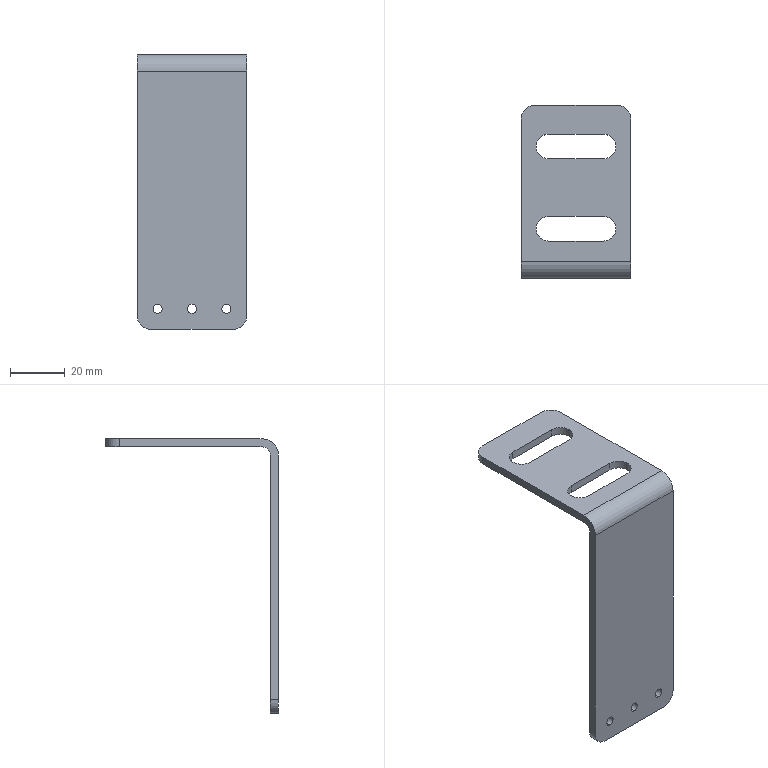Part | STEP file | 1 solid | 30 faces | box 40 x 63 x 100 mm | volume 17364 mm3 | cylinder 16 | plane 12 | cone 2 | commonest cylinder face diameters 3.3 x6 9 x4 10 x4 6 x1 12 x1